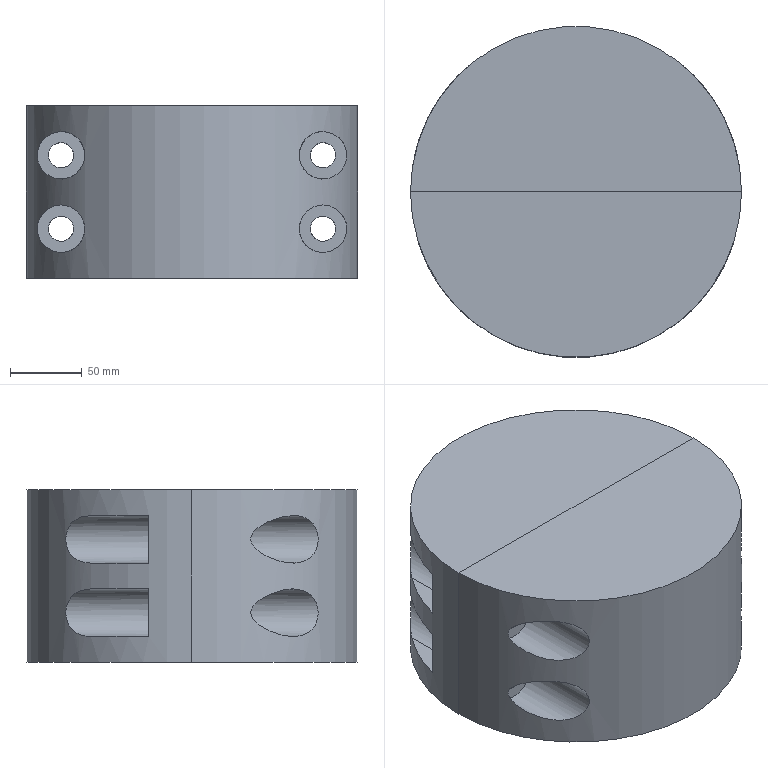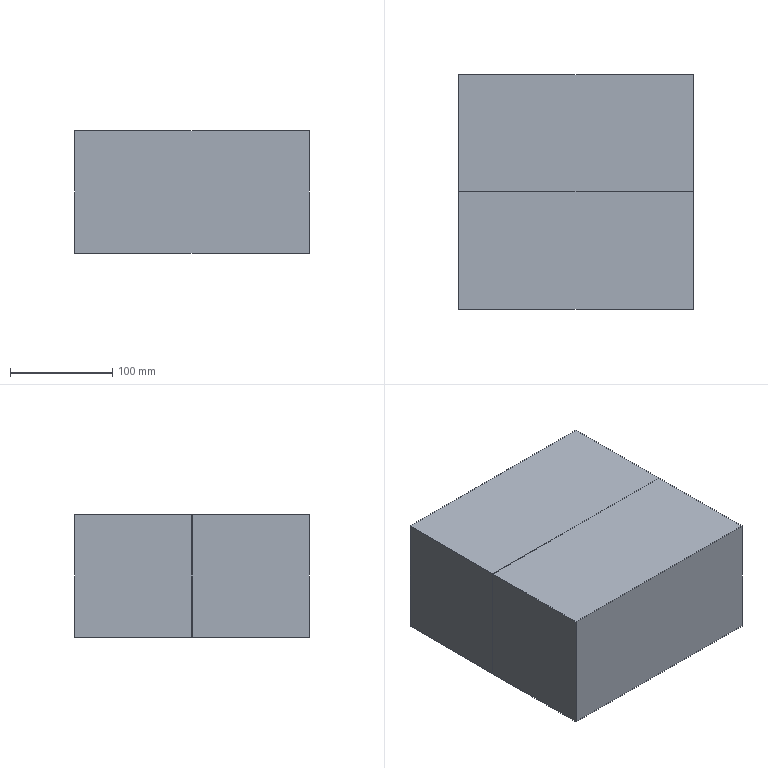CAM job | NX | 3-axis milling, drilling | part box 230 x 230 x 120 mm | stock box 230 x 230 x 120 mm
Tools:
number,name,description,diameter,corner_radius,flute_length,length,flutes
1,D25,Milling Tool-5 Parameters,25.0,0.0,50.0,75.0,2
2,ZXZ,Milling Tool-5 Parameters,6.0,0.0,50.0,75.0,2
3,21.5ZT,Drilling Tool,21.5,0.0,35.0,50.0,2
4,17.5ZT,Drilling Tool,17.5,0.0,35.0,50.0,2
5,D15XYD,Thread Mill,15.0,0.0,2.5,50.0,2
Operations:
program,operation,operation_type,tool,method,geometry_group,spindle_rpm,surface_speed,feed_per_tooth,feed_cut,feed_plunge,cut_length_mm,path_length_mm,cut_time_min,machine_time_min
1,ZLEVEL_PROFILE,ZLevelMilling,D25,METHOD,A,1000.0,78.0,1.0,2000.0,100.0,39736.111,41061.564,19.868,20.001
1,DRILLING,Operation,ZXZ,METHOD,A,3500.0,65.0,0.0357,250.0,0.0,16.0,555.201,0.064,0.1179
1,DRILLING_COPY,Operation,21.5ZT,METHOD,A,500.0,33.0,0.08,80.0,0.0,175.837,874.875,2.198,2.268
2,DRILLING_COPY_1_1,Operation,ZXZ,METHOD,B,3500.0,65.0,0.0357,250.0,0.0,16.0,385.201,0.064,0.1009
2,DRILLING_COPY_COPY,Operation,17.5ZT,METHOD,B,500.0,33.0,0.08,80.0,0.0,173.03,699.261,2.163,2.216
2,THREAD_MILLING,ThreadMilling,D15XYD,METHOD,B,1200.0,56.0,0.2083,500.0,100.0,2658.41,3552.619,5.317,5.406
2,THREAD_MILLING_COPY,ThreadMilling,D15XYD,METHOD,B,1200.0,56.0,0.2083,500.0,100.0,1044.528,1686.528,2.089,2.153